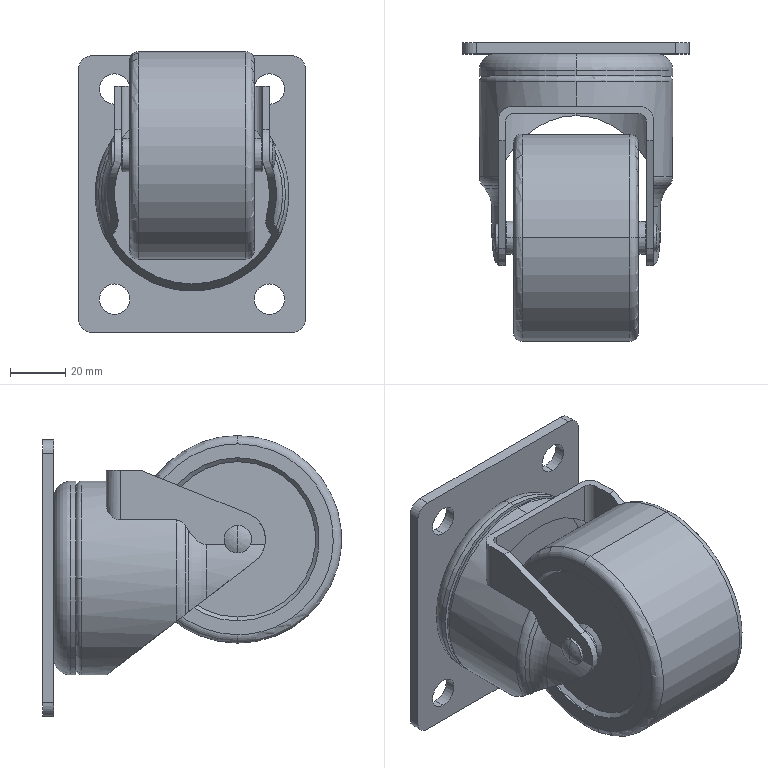Part | SolidWorks | 3 solids | 108 faces | box 82 x 108 x 101.5 mm | volume 268701 mm3 | cylinder 44 | plane 26 | torus 18 | cone 16 | spline 4 | commonest cylinder face diameters 10 x10 11 x8 70 x6 12 x4 59 x4 6 x2